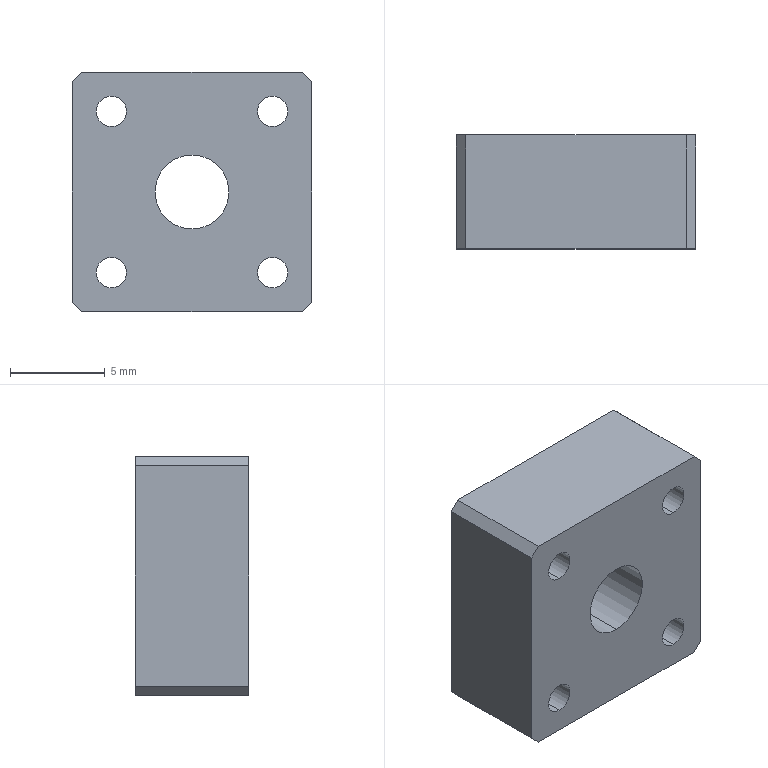Part | SolidWorks | features Extrusion 1, HoleWzd 1 | 1 solid | 20 faces | box 12.63 x 6 x 12.63 mm | volume 834.171 mm3 | cylinder 10 | plane 10 | commonest cylinder face diameters 1.6 x8 3.9 x2
STEP:
#1=CARTESIAN_POINT('',(-4.25,0.,-5.05));
#2=VERTEX_POINT('',#1);
#3=CARTESIAN_POINT('',(-4.25,0.,-3.45));
#4=VERTEX_POINT('',#3);
#5=CARTESIAN_POINT('',(-4.25,0.,-4.25));
#6=DIRECTION('',(0.,1.,0.));
#7=DIRECTION('',(0.,0.,1.));
#8=AXIS2_PLACEMENT_3D('',#5,#6,#7);
#9=CIRCLE('',#8,0.8);
#10=EDGE_CURVE('',#2,#4,#9,.T.);
#11=ORIENTED_EDGE('',*,*,#10,.F.);
#12=CARTESIAN_POINT('',(-4.25,6.,-5.05));
#13=VERTEX_POINT('',#12);
#14=CARTESIAN_POINT('',(-4.25,6.,-5.05));
#15=DIRECTION('',(0.,1.,0.));
#16=VECTOR('',#15,1000.);
#17=LINE('',#14,#16);
#18=EDGE_CURVE('',#2,#13,#17,.T.);
#19=ORIENTED_EDGE('',*,*,#18,.T.);
#20=CARTESIAN_POINT('',(-4.25,6.,-3.45));
#21=VERTEX_POINT('',#20);
#22=CARTESIAN_POINT('',(-4.25,6.,-4.25));
#23=DIRECTION('',(0.,1.,0.));
#24=DIRECTION('',(0.,0.,1.));
#25=AXIS2_PLACEMENT_3D('',#22,#23,#24);
#26=CIRCLE('',#25,0.8);
#27=EDGE_CURVE('',#13,#21,#26,.T.);
#28=ORIENTED_EDGE('',*,*,#27,.T.);
#29=CARTESIAN_POINT('',(-4.25,6.,-3.45));
#30=DIRECTION('',(0.,1.,0.));
#31=VECTOR('',#30,1000.);
#32=LINE('',#29,#31);
#33=EDGE_CURVE('',#4,#21,#32,.T.);
#34=ORIENTED_EDGE('',*,*,#33,.F.);
#35=EDGE_LOOP('',(#11,#19,#28,#34));
#36=FACE_OUTER_BOUND('',#35,.T.);
#37=CARTESIAN_POINT('',(-4.25,6.,-4.25));
#38=DIRECTION('',(0.,1.,0.));
#39=DIRECTION('',(0.,0.,1.));
#40=AXIS2_PLACEMENT_3D('',#37,#38,#39);
#41=CYLINDRICAL_SURFACE('',#40,0.8);
#42=ADVANCED_FACE('',(#36),#41,.F.);
#43=CARTESIAN_POINT('',(4.25,0.,-5.05));
#44=VERTEX_POINT('',#43);
#45=CARTESIAN_POINT('',(4.25,0.,-3.45));
#46=VERTEX_POINT('',#45);
#47=CARTESIAN_POINT('',(4.25,0.,-4.25));
#48=DIRECTION('',(0.,1.,0.));
#49=DIRECTION('',(0.,0.,1.));
#50=AXIS2_PLACEMENT_3D('',#47,#48,#49);
#51=CIRCLE('',#50,0.8);
#52=EDGE_CURVE('',#44,#46,#51,.T.);
#53=ORIENTED_EDGE('',*,*,#52,.F.);
#54=CARTESIAN_POINT('',(4.25,6.,-5.05));
#55=VERTEX_POINT('',#54);
#56=CARTESIAN_POINT('',(4.25,6.,-5.05));
#57=DIRECTION('',(0.,1.,0.));
#58=VECTOR('',#57,1000.);
#59=LINE('',#56,#58);
#60=EDGE_CURVE('',#44,#55,#59,.T.);
#61=ORIENTED_EDGE('',*,*,#60,.T.);
#62=CARTESIAN_POINT('',(4.25,6.,-3.45));
#63=VERTEX_POINT('',#62);
#64=CARTESIAN_POINT('',(4.25,6.,-4.25));
#65=DIRECTION('',(0.,1.,0.));
#66=DIRECTION('',(0.,0.,1.));
#67=AXIS2_PLACEMENT_3D('',#64,#65,#66);
#68=CIRCLE('',#67,0.8);
#69=EDGE_CURVE('',#55,#63,#68,.T.);
#70=ORIENTED_EDGE('',*,*,#69,.T.);
#71=CARTESIAN_POINT('',(4.25,6.,-3.45));
#72=DIRECTION('',(0.,1.,0.));
#73=VECTOR('',#72,1000.);
#74=LINE('',#71,#73);
#75=EDGE_CURVE('',#46,#63,#74,.T.);
#76=ORIENTED_EDGE('',*,*,#75,.F.);
#77=EDGE_LOOP('',(#53,#61,#70,#76));
#78=FACE_OUTER_BOUND('',#77,.T.);
#79=CARTESIAN_POINT('',(4.25,6.,-4.25));
#80=DIRECTION('',(0.,1.,0.));
#81=DIRECTION('',(0.,0.,1.));
#82=AXIS2_PLACEMENT_3D('',#79,#80,#81);
#83=CYLINDRICAL_SURFACE('',#82,0.8);
#84=ADVANCED_FACE('',(#78),#83,.F.);
#85=CARTESIAN_POINT('',(4.25,0.,3.45));
#86=VERTEX_POINT('',#85);
#87=CARTESIAN_POINT('',(4.25,0.,5.05));
#88=VERTEX_POINT('',#87);
#89=CARTESIAN_POINT('',(4.25,0.,4.25));
#90=DIRECTION('',(0.,1.,0.));
#91=DIRECTION('',(0.,0.,1.));
#92=AXIS2_PLACEMENT_3D('',#89,#90,#91);
#93=CIRCLE('',#92,0.8);
#94=EDGE_CURVE('',#86,#88,#93,.T.);
#95=ORIENTED_EDGE('',*,*,#94,.F.);
#96=CARTESIAN_POINT('',(4.25,6.,3.45));
#97=VERTEX_POINT('',#96);
#98=CARTESIAN_POINT('',(4.25,6.,3.45));
#99=DIRECTION('',(0.,1.,0.));
#100=VECTOR('',#99,1000.);
#101=LINE('',#98,#100);
#102=EDGE_CURVE('',#86,#97,#101,.T.);
#103=ORIENTED_EDGE('',*,*,#102,.T.);
#104=CARTESIAN_POINT('',(4.25,6.,5.05));
#105=VERTEX_POINT('',#104);
#106=CARTESIAN_POINT('',(4.25,6.,4.25));
#107=DIRECTION('',(0.,1.,0.));
#108=DIRECTION('',(0.,0.,1.));
#109=AXIS2_PLACEMENT_3D('',#106,#107,#108);
#110=CIRCLE('',#109,0.8);
#111=EDGE_CURVE('',#97,#105,#110,.T.);
#112=ORIENTED_EDGE('',*,*,#111,.T.);
#113=CARTESIAN_POINT('',(4.25,6.,5.05));
#114=DIRECTION('',(0.,1.,0.));
#115=VECTOR('',#114,1000.);
#116=LINE('',#113,#115);
#117=EDGE_CURVE('',#88,#105,#116,.T.);
#118=ORIENTED_EDGE('',*,*,#117,.F.);
#119=EDGE_LOOP('',(#95,#103,#112,#118));
#120=FACE_OUTER_BOUND('',#119,.T.);
#121=CARTESIAN_POINT('',(4.25,6.,4.25));
#122=DIRECTION('',(0.,1.,0.));
#123=DIRECTION('',(0.,0.,1.));
#124=AXIS2_PLACEMENT_3D('',#121,#122,#123);
#125=CYLINDRICAL_SURFACE('',#124,0.8);
#126=ADVANCED_FACE('',(#120),#125,.F.);
#127=CARTESIAN_POINT('',(-4.25,0.,3.45));
#128=VERTEX_POINT('',#127);
#129=CARTESIAN_POINT('',(-4.25,0.,5.05));
#130=VERTEX_POINT('',#129);
#131=CARTESIAN_POINT('',(-4.25,0.,4.25));
#132=DIRECTION('',(0.,1.,0.));
#133=DIRECTION('',(0.,0.,1.));
#134=AXIS2_PLACEMENT_3D('',#131,#132,#133);
#135=CIRCLE('',#134,0.8);
#136=EDGE_CURVE('',#128,#130,#135,.T.);
#137=ORIENTED_EDGE('',*,*,#136,.F.);
#138=CARTESIAN_POINT('',(-4.25,6.,3.45));
#139=VERTEX_POINT('',#138);
#140=CARTESIAN_POINT('',(-4.25,6.,3.45));
#141=DIRECTION('',(0.,1.,0.));
#142=VECTOR('',#141,1000.);
#143=LINE('',#140,#142);
#144=EDGE_CURVE('',#128,#139,#143,.T.);
#145=ORIENTED_EDGE('',*,*,#144,.T.);
#146=CARTESIAN_POINT('',(-4.25,6.,5.05));
#147=VERTEX_POINT('',#146);
#148=CARTESIAN_POINT('',(-4.25,6.,4.25));
#149=DIRECTION('',(0.,1.,0.));
#150=DIRECTION('',(0.,0.,1.));
#151=AXIS2_PLACEMENT_3D('',#148,#149,#150);
#152=CIRCLE('',#151,0.8);
#153=EDGE_CURVE('',#139,#147,#152,.T.);
#154=ORIENTED_EDGE('',*,*,#153,.T.);
#155=CARTESIAN_POINT('',(-4.25,6.,5.05));
#156=DIRECTION('',(0.,1.,0.));
#157=VECTOR('',#156,1000.);
#158=LINE('',#155,#157);
#159=EDGE_CURVE('',#130,#147,#158,.T.);
#160=ORIENTED_EDGE('',*,*,#159,.F.);
#161=EDGE_LOOP('',(#137,#145,#154,#160));
#162=FACE_OUTER_BOUND('',#161,.T.);
#163=CARTESIAN_POINT('',(-4.25,6.,4.25));
#164=DIRECTION('',(0.,1.,0.));
#165=DIRECTION('',(0.,0.,1.));
#166=AXIS2_PLACEMENT_3D('',#163,#164,#165);
#167=CYLINDRICAL_SURFACE('',#166,0.8);
#168=ADVANCED_FACE('',(#162),#167,.F.);
#169=CARTESIAN_POINT('',(0.,6.,-1.95));
#170=VERTEX_POINT('',#169);
#171=CARTESIAN_POINT('',(0.,6.,1.95));
#172=VERTEX_POINT('',#171);
#173=CARTESIAN_POINT('',(0.,6.,0.));
#174=DIRECTION('',(0.,1.,0.));
#175=DIRECTION('',(0.,0.,1.));
#176=AXIS2_PLACEMENT_3D('',#173,#174,#175);
#177=CIRCLE('',#176,1.95);
#178=EDGE_CURVE('',#170,#172,#177,.T.);
#179=ORIENTED_EDGE('',*,*,#178,.T.);
#180=CARTESIAN_POINT('',(0.,0.,1.95));
#181=VERTEX_POINT('',#180);
#182=CARTESIAN_POINT('',(0.,6.,1.95));
#183=DIRECTION('',(0.,-1.,0.));
#184=VECTOR('',#183,1000.);
#185=LINE('',#182,#184);
#186=EDGE_CURVE('',#172,#181,#185,.T.);
#187=ORIENTED_EDGE('',*,*,#186,.T.);
#188=CARTESIAN_POINT('',(0.,0.,-1.95));
#189=VERTEX_POINT('',#188);
#190=CARTESIAN_POINT('',(0.,0.,0.));
#191=DIRECTION('',(0.,1.,0.));
#192=DIRECTION('',(0.,0.,1.));
#193=AXIS2_PLACEMENT_3D('',#190,#191,#192);
#194=CIRCLE('',#193,1.95);
#195=EDGE_CURVE('',#189,#181,#194,.T.);
#196=ORIENTED_EDGE('',*,*,#195,.F.);
#197=CARTESIAN_POINT('',(0.,6.,-1.95));
#198=DIRECTION('',(0.,-1.,0.));
#199=VECTOR('',#198,1000.);
#200=LINE('',#197,#199);
#201=EDGE_CURVE('',#170,#189,#200,.T.);
#202=ORIENTED_EDGE('',*,*,#201,.F.);
#203=EDGE_LOOP('',(#179,#187,#196,#202));
#204=FACE_OUTER_BOUND('',#203,.T.);
#205=CARTESIAN_POINT('',(0.,6.,0.));
#206=DIRECTION('',(0.,-1.,0.));
#207=DIRECTION('',(0.,0.,-1.));
#208=AXIS2_PLACEMENT_3D('',#205,#206,#207);
#209=CYLINDRICAL_SURFACE('',#208,1.95);
#210=ADVANCED_FACE('',(#204),#209,.F.);
#211=CARTESIAN_POINT('',(-4.25,6.,-4.25));
#212=DIRECTION('',(0.,1.,0.));
#213=DIRECTION('',(0.,0.,1.));
#214=AXIS2_PLACEMENT_3D('',#211,#212,#213);
#215=CIRCLE('',#214,0.8);
#216=EDGE_CURVE('',#21,#13,#215,.T.);
#217=ORIENTED_EDGE('',*,*,#216,.F.);
#218=ORIENTED_EDGE('',*,*,#27,.F.);
#219=EDGE_LOOP('',(#217,#218));
#220=FACE_BOUND('',#219,.T.);
#221=CARTESIAN_POINT('',(4.25,6.,-4.25));
#222=DIRECTION('',(0.,1.,0.));
#223=DIRECTION('',(0.,0.,1.));
#224=AXIS2_PLACEMENT_3D('',#221,#222,#223);
#225=CIRCLE('',#224,0.8);
#226=EDGE_CURVE('',#63,#55,#225,.T.);
#227=ORIENTED_EDGE('',*,*,#226,.F.);
#228=ORIENTED_EDGE('',*,*,#69,.F.);
#229=EDGE_LOOP('',(#227,#228));
#230=FACE_BOUND('',#229,.T.);
#231=CARTESIAN_POINT('',(4.25,6.,4.25));
#232=DIRECTION('',(0.,1.,0.));
#233=DIRECTION('',(0.,0.,1.));
#234=AXIS2_PLACEMENT_3D('',#231,#232,#233);
#235=CIRCLE('',#234,0.8);
#236=EDGE_CURVE('',#105,#97,#235,.T.);
#237=ORIENTED_EDGE('',*,*,#236,.F.);
#238=ORIENTED_EDGE('',*,*,#111,.F.);
#239=EDGE_LOOP('',(#237,#238));
#240=FACE_BOUND('',#239,.T.);
#241=CARTESIAN_POINT('',(-4.25,6.,4.25));
#242=DIRECTION('',(0.,1.,0.));
#243=DIRECTION('',(0.,0.,1.));
#244=AXIS2_PLACEMENT_3D('',#241,#242,#243);
#245=CIRCLE('',#244,0.8);
#246=EDGE_CURVE('',#147,#139,#245,.T.);
#247=ORIENTED_EDGE('',*,*,#246,.F.);
#248=ORIENTED_EDGE('',*,*,#153,.F.);
#249=EDGE_LOOP('',(#247,#248));
#250=FACE_BOUND('',#249,.T.);
#251=CARTESIAN_POINT('',(-6.315,6.,-5.815));
#252=VERTEX_POINT('',#251);
#253=CARTESIAN_POINT('',(-6.315,6.,5.815));
#254=VERTEX_POINT('',#253);
#255=CARTESIAN_POINT('',(-6.315,6.,5.815));
#256=DIRECTION('',(0.,0.,1.));
#257=VECTOR('',#256,1000.);
#258=LINE('',#255,#257);
#259=EDGE_CURVE('',#252,#254,#258,.T.);
#260=ORIENTED_EDGE('',*,*,#259,.T.);
#261=CARTESIAN_POINT('',(-5.815,6.,6.315));
#262=VERTEX_POINT('',#261);
#263=CARTESIAN_POINT('',(-6.315,6.,5.815));
#264=DIRECTION('',(0.7071,0.,0.7071));
#265=VECTOR('',#264,1000.);
#266=LINE('',#263,#265);
#267=EDGE_CURVE('',#254,#262,#266,.T.);
#268=ORIENTED_EDGE('',*,*,#267,.T.);
#269=CARTESIAN_POINT('',(5.815,6.,6.315));
#270=VERTEX_POINT('',#269);
#271=CARTESIAN_POINT('',(-5.815,6.,6.315));
#272=DIRECTION('',(1.,0.,0.));
#273=VECTOR('',#272,1000.);
#274=LINE('',#271,#273);
#275=EDGE_CURVE('',#262,#270,#274,.T.);
#276=ORIENTED_EDGE('',*,*,#275,.T.);
#277=CARTESIAN_POINT('',(6.315,6.,5.815));
#278=VERTEX_POINT('',#277);
#279=CARTESIAN_POINT('',(5.815,6.,6.315));
#280=DIRECTION('',(0.7071,0.,-0.7071));
#281=VECTOR('',#280,1000.);
#282=LINE('',#279,#281);
#283=EDGE_CURVE('',#270,#278,#282,.T.);
#284=ORIENTED_EDGE('',*,*,#283,.T.);
#285=CARTESIAN_POINT('',(6.315,6.,-5.815));
#286=VERTEX_POINT('',#285);
#287=CARTESIAN_POINT('',(6.315,6.,5.815));
#288=DIRECTION('',(0.,0.,-1.));
#289=VECTOR('',#288,1000.);
#290=LINE('',#287,#289);
#291=EDGE_CURVE('',#278,#286,#290,.T.);
#292=ORIENTED_EDGE('',*,*,#291,.T.);
#293=CARTESIAN_POINT('',(5.815,6.,-6.315));
#294=VERTEX_POINT('',#293);
#295=CARTESIAN_POINT('',(5.815,6.,-6.315));
#296=DIRECTION('',(-0.7071,0.,-0.7071));
#297=VECTOR('',#296,1000.);
#298=LINE('',#295,#297);
#299=EDGE_CURVE('',#286,#294,#298,.T.);
#300=ORIENTED_EDGE('',*,*,#299,.T.);
#301=CARTESIAN_POINT('',(-5.815,6.,-6.315));
#302=VERTEX_POINT('',#301);
#303=CARTESIAN_POINT('',(-5.815,6.,-6.315));
#304=DIRECTION('',(-1.,0.,0.));
#305=VECTOR('',#304,1000.);
#306=LINE('',#303,#305);
#307=EDGE_CURVE('',#294,#302,#306,.T.);
#308=ORIENTED_EDGE('',*,*,#307,.T.);
#309=CARTESIAN_POINT('',(-6.315,6.,-5.815));
#310=DIRECTION('',(-0.7071,0.,0.7071));
#311=VECTOR('',#310,1000.);
#312=LINE('',#309,#311);
#313=EDGE_CURVE('',#302,#252,#312,.T.);
#314=ORIENTED_EDGE('',*,*,#313,.T.);
#315=EDGE_LOOP('',(#260,#268,#276,#284,#292,#300,#308,#314));
#316=FACE_OUTER_BOUND('',#315,.T.);
#317=ORIENTED_EDGE('',*,*,#178,.F.);
#318=CARTESIAN_POINT('',(0.,6.,0.));
#319=DIRECTION('',(0.,1.,0.));
#320=DIRECTION('',(0.,0.,1.));
#321=AXIS2_PLACEMENT_3D('',#318,#319,#320);
#322=CIRCLE('',#321,1.95);
#323=EDGE_CURVE('',#172,#170,#322,.T.);
#324=ORIENTED_EDGE('',*,*,#323,.F.);
#325=EDGE_LOOP('',(#317,#324));
#326=FACE_BOUND('',#325,.T.);
#327=CARTESIAN_POINT('',(-6.315,6.,-6.315));
#328=DIRECTION('',(0.,-1.,0.));
#329=DIRECTION('',(0.,0.,-1.));
#330=AXIS2_PLACEMENT_3D('',#327,#328,#329);
#331=PLANE('',#330);
#332=ADVANCED_FACE('',(#220,#230,#240,#250,#316,#326),#331,.F.);
#333=CARTESIAN_POINT('',(-4.25,0.,-4.25));
#334=DIRECTION('',(0.,1.,0.));
#335=DIRECTION('',(0.,0.,1.));
#336=AXIS2_PLACEMENT_3D('',#333,#334,#335);
#337=CIRCLE('',#336,0.8);
#338=EDGE_CURVE('',#4,#2,#337,.T.);
#339=ORIENTED_EDGE('',*,*,#338,.T.);
#340=ORIENTED_EDGE('',*,*,#10,.T.);
#341=EDGE_LOOP('',(#339,#340));
#342=FACE_BOUND('',#341,.T.);
#343=CARTESIAN_POINT('',(4.25,0.,-4.25));
#344=DIRECTION('',(0.,1.,0.));
#345=DIRECTION('',(0.,0.,1.));
#346=AXIS2_PLACEMENT_3D('',#343,#344,#345);
#347=CIRCLE('',#346,0.8);
#348=EDGE_CURVE('',#46,#44,#347,.T.);
#349=ORIENTED_EDGE('',*,*,#348,.T.);
#350=ORIENTED_EDGE('',*,*,#52,.T.);
#351=EDGE_LOOP('',(#349,#350));
#352=FACE_BOUND('',#351,.T.);
#353=CARTESIAN_POINT('',(4.25,0.,4.25));
#354=DIRECTION('',(0.,1.,0.));
#355=DIRECTION('',(0.,0.,1.));
#356=AXIS2_PLACEMENT_3D('',#353,#354,#355);
#357=CIRCLE('',#356,0.8);
#358=EDGE_CURVE('',#88,#86,#357,.T.);
#359=ORIENTED_EDGE('',*,*,#358,.T.);
#360=ORIENTED_EDGE('',*,*,#94,.T.);
#361=EDGE_LOOP('',(#359,#360));
#362=FACE_BOUND('',#361,.T.);
#363=CARTESIAN_POINT('',(-4.25,0.,4.25));
#364=DIRECTION('',(0.,1.,0.));
#365=DIRECTION('',(0.,0.,1.));
#366=AXIS2_PLACEMENT_3D('',#363,#364,#365);
#367=CIRCLE('',#366,0.8);
#368=EDGE_CURVE('',#130,#128,#367,.T.);
#369=ORIENTED_EDGE('',*,*,#368,.T.);
#370=ORIENTED_EDGE('',*,*,#136,.T.);
#371=EDGE_LOOP('',(#369,#370));
#372=FACE_BOUND('',#371,.T.);
#373=CARTESIAN_POINT('',(-6.315,0.,-5.815));
#374=VERTEX_POINT('',#373);
#375=CARTESIAN_POINT('',(-6.315,0.,5.815));
#376=VERTEX_POINT('',#375);
#377=CARTESIAN_POINT('',(-6.315,0.,5.815));
#378=DIRECTION('',(0.,0.,1.));
#379=VECTOR('',#378,1000.);
#380=LINE('',#377,#379);
#381=EDGE_CURVE('',#374,#376,#380,.T.);
#382=ORIENTED_EDGE('',*,*,#381,.F.);
#383=CARTESIAN_POINT('',(-5.815,0.,-6.315));
#384=VERTEX_POINT('',#383);
#385=CARTESIAN_POINT('',(-6.315,0.,-5.815));
#386=DIRECTION('',(-0.7071,0.,0.7071));
#387=VECTOR('',#386,1000.);
#388=LINE('',#385,#387);
#389=EDGE_CURVE('',#384,#374,#388,.T.);
#390=ORIENTED_EDGE('',*,*,#389,.F.);
#391=CARTESIAN_POINT('',(5.815,0.,-6.315));
#392=VERTEX_POINT('',#391);
#393=CARTESIAN_POINT('',(-5.815,0.,-6.315));
#394=DIRECTION('',(-1.,0.,0.));
#395=VECTOR('',#394,1000.);
#396=LINE('',#393,#395);
#397=EDGE_CURVE('',#392,#384,#396,.T.);
#398=ORIENTED_EDGE('',*,*,#397,.F.);
#399=CARTESIAN_POINT('',(6.315,0.,-5.815));
#400=VERTEX_POINT('',#399);
#401=CARTESIAN_POINT('',(5.815,0.,-6.315));
#402=DIRECTION('',(-0.7071,0.,-0.7071));
#403=VECTOR('',#402,1000.);
#404=LINE('',#401,#403);
#405=EDGE_CURVE('',#400,#392,#404,.T.);
#406=ORIENTED_EDGE('',*,*,#405,.F.);
#407=CARTESIAN_POINT('',(6.315,0.,5.815));
#408=VERTEX_POINT('',#407);
#409=CARTESIAN_POINT('',(6.315,0.,5.815));
#410=DIRECTION('',(0.,0.,-1.));
#411=VECTOR('',#410,1000.);
#412=LINE('',#409,#411);
#413=EDGE_CURVE('',#408,#400,#412,.T.);
#414=ORIENTED_EDGE('',*,*,#413,.F.);
#415=CARTESIAN_POINT('',(5.815,0.,6.315));
#416=VERTEX_POINT('',#415);
#417=CARTESIAN_POINT('',(5.815,0.,6.315));
#418=DIRECTION('',(0.7071,0.,-0.7071));
#419=VECTOR('',#418,1000.);
#420=LINE('',#417,#419);
#421=EDGE_CURVE('',#416,#408,#420,.T.);
#422=ORIENTED_EDGE('',*,*,#421,.F.);
#423=CARTESIAN_POINT('',(-5.815,0.,6.315));
#424=VERTEX_POINT('',#423);
#425=CARTESIAN_POINT('',(-5.815,0.,6.315));
#426=DIRECTION('',(1.,0.,0.));
#427=VECTOR('',#426,1000.);
#428=LINE('',#425,#427);
#429=EDGE_CURVE('',#424,#416,#428,.T.);
#430=ORIENTED_EDGE('',*,*,#429,.F.);
#431=CARTESIAN_POINT('',(-6.315,0.,5.815));
#432=DIRECTION('',(0.7071,0.,0.7071));
#433=VECTOR('',#432,1000.);
#434=LINE('',#431,#433);
#435=EDGE_CURVE('',#376,#424,#434,.T.);
#436=ORIENTED_EDGE('',*,*,#435,.F.);
#437=EDGE_LOOP('',(#382,#390,#398,#406,#414,#422,#430,#436));
#438=FACE_OUTER_BOUND('',#437,.T.);
#439=ORIENTED_EDGE('',*,*,#195,.T.);
#440=CARTESIAN_POINT('',(0.,0.,0.));
#441=DIRECTION('',(0.,1.,0.));
#442=DIRECTION('',(0.,0.,1.));
#443=AXIS2_PLACEMENT_3D('',#440,#441,#442);
#444=CIRCLE('',#443,1.95);
#445=EDGE_CURVE('',#181,#189,#444,.T.);
#446=ORIENTED_EDGE('',*,*,#445,.T.);
#447=EDGE_LOOP('',(#439,#446));
#448=FACE_BOUND('',#447,.T.);
#449=CARTESIAN_POINT('',(-6.315,0.,-6.315));
#450=DIRECTION('',(0.,-1.,0.));
#451=DIRECTION('',(0.,0.,-1.));
#452=AXIS2_PLACEMENT_3D('',#449,#450,#451);
#453=PLANE('',#452);
#454=ADVANCED_FACE('',(#342,#352,#362,#372,#438,#448),#453,.T.);
#455=ORIENTED_EDGE('',*,*,#381,.T.);
#456=CARTESIAN_POINT('',(-6.315,6.,5.815));
#457=DIRECTION('',(0.,-1.,0.));
#458=VECTOR('',#457,1000.);
#459=LINE('',#456,#458);
#460=EDGE_CURVE('',#254,#376,#459,.T.);
#461=ORIENTED_EDGE('',*,*,#460,.F.);
#462=ORIENTED_EDGE('',*,*,#259,.F.);
#463=CARTESIAN_POINT('',(-6.315,6.,-5.815));
#464=DIRECTION('',(0.,-1.,0.));
#465=VECTOR('',#464,1000.);
#466=LINE('',#463,#465);
#467=EDGE_CURVE('',#252,#374,#466,.T.);
#468=ORIENTED_EDGE('',*,*,#467,.T.);
#469=EDGE_LOOP('',(#455,#461,#462,#468));
#470=FACE_OUTER_BOUND('',#469,.T.);
#471=CARTESIAN_POINT('',(-6.315,6.,5.815));
#472=DIRECTION('',(1.,0.,0.));
#473=DIRECTION('',(0.,0.,-1.));
#474=AXIS2_PLACEMENT_3D('',#471,#472,#473);
#475=PLANE('',#474);
#476=ADVANCED_FACE('',(#470),#475,.F.);
#477=ORIENTED_EDGE('',*,*,#435,.T.);
#478=CARTESIAN_POINT('',(-5.815,6.,6.315));
#479=DIRECTION('',(0.,-1.,0.));
#480=VECTOR('',#479,1000.);
#481=LINE('',#478,#480);
#482=EDGE_CURVE('',#262,#424,#481,.T.);
#483=ORIENTED_EDGE('',*,*,#482,.F.);
#484=ORIENTED_EDGE('',*,*,#267,.F.);
#485=ORIENTED_EDGE('',*,*,#460,.T.);
#486=EDGE_LOOP('',(#477,#483,#484,#485));
#487=FACE_OUTER_BOUND('',#486,.T.);
#488=CARTESIAN_POINT('',(-6.315,6.,5.815));
#489=DIRECTION('',(0.7071,0.,-0.7071));
#490=DIRECTION('',(-0.7071,0.,-0.7071));
#491=AXIS2_PLACEMENT_3D('',#488,#489,#490);
#492=PLANE('',#491);
#493=ADVANCED_FACE('',(#487),#492,.F.);
#494=ORIENTED_EDGE('',*,*,#429,.T.);
#495=CARTESIAN_POINT('',(5.815,6.,6.315));
#496=DIRECTION('',(0.,-1.,0.));
#497=VECTOR('',#496,1000.);
#498=LINE('',#495,#497);
#499=EDGE_CURVE('',#270,#416,#498,.T.);
#500=ORIENTED_EDGE('',*,*,#499,.F.);
#501=ORIENTED_EDGE('',*,*,#275,.F.);
#502=ORIENTED_EDGE('',*,*,#482,.T.);
#503=EDGE_LOOP('',(#494,#500,#501,#502));
#504=FACE_OUTER_BOUND('',#503,.T.);
#505=CARTESIAN_POINT('',(-5.815,6.,6.315));
#506=DIRECTION('',(0.,0.,-1.));
#507=DIRECTION('',(-1.,0.,0.));
#508=AXIS2_PLACEMENT_3D('',#505,#506,#507);
#509=PLANE('',#508);
#510=ADVANCED_FACE('',(#504),#509,.F.);
#511=ORIENTED_EDGE('',*,*,#421,.T.);
#512=CARTESIAN_POINT('',(6.315,6.,5.815));
#513=DIRECTION('',(0.,-1.,0.));
#514=VECTOR('',#513,1000.);
#515=LINE('',#512,#514);
#516=EDGE_CURVE('',#278,#408,#515,.T.);
#517=ORIENTED_EDGE('',*,*,#516,.F.);
#518=ORIENTED_EDGE('',*,*,#283,.F.);
#519=ORIENTED_EDGE('',*,*,#499,.T.);
#520=EDGE_LOOP('',(#511,#517,#518,#519));
#521=FACE_OUTER_BOUND('',#520,.T.);
#522=CARTESIAN_POINT('',(5.815,6.,6.315));
#523=DIRECTION('',(-0.7071,0.,-0.7071));
#524=DIRECTION('',(-0.7071,0.,0.7071));
#525=AXIS2_PLACEMENT_3D('',#522,#523,#524);
#526=PLANE('',#525);
#527=ADVANCED_FACE('',(#521),#526,.F.);
#528=ORIENTED_EDGE('',*,*,#413,.T.);
#529=CARTESIAN_POINT('',(6.315,6.,-5.815));
#530=DIRECTION('',(0.,-1.,0.));
#531=VECTOR('',#530,1000.);
#532=LINE('',#529,#531);
#533=EDGE_CURVE('',#286,#400,#532,.T.);
#534=ORIENTED_EDGE('',*,*,#533,.F.);
#535=ORIENTED_EDGE('',*,*,#291,.F.);
#536=ORIENTED_EDGE('',*,*,#516,.T.);
#537=EDGE_LOOP('',(#528,#534,#535,#536));
#538=FACE_OUTER_BOUND('',#537,.T.);
#539=CARTESIAN_POINT('',(6.315,6.,5.815));
#540=DIRECTION('',(-1.,0.,0.));
#541=DIRECTION('',(0.,0.,1.));
#542=AXIS2_PLACEMENT_3D('',#539,#540,#541);
#543=PLANE('',#542);
#544=ADVANCED_FACE('',(#538),#543,.F.);
#545=ORIENTED_EDGE('',*,*,#405,.T.);
#546=CARTESIAN_POINT('',(5.815,6.,-6.315));
#547=DIRECTION('',(0.,-1.,0.));
#548=VECTOR('',#547,1000.);
#549=LINE('',#546,#548);
#550=EDGE_CURVE('',#294,#392,#549,.T.);
#551=ORIENTED_EDGE('',*,*,#550,.F.);
#552=ORIENTED_EDGE('',*,*,#299,.F.);
#553=ORIENTED_EDGE('',*,*,#533,.T.);
#554=EDGE_LOOP('',(#545,#551,#552,#553));
#555=FACE_OUTER_BOUND('',#554,.T.);
#556=CARTESIAN_POINT('',(5.815,6.,-6.315));
#557=DIRECTION('',(-0.7071,0.,0.7071));
#558=DIRECTION('',(0.7071,0.,0.7071));
#559=AXIS2_PLACEMENT_3D('',#556,#557,#558);
#560=PLANE('',#559);
#561=ADVANCED_FACE('',(#555),#560,.F.);
#562=ORIENTED_EDGE('',*,*,#397,.T.);
#563=CARTESIAN_POINT('',(-5.815,6.,-6.315));
#564=DIRECTION('',(0.,-1.,0.));
#565=VECTOR('',#564,1000.);
#566=LINE('',#563,#565);
#567=EDGE_CURVE('',#302,#384,#566,.T.);
#568=ORIENTED_EDGE('',*,*,#567,.F.);
#569=ORIENTED_EDGE('',*,*,#307,.F.);
#570=ORIENTED_EDGE('',*,*,#550,.T.);
#571=EDGE_LOOP('',(#562,#568,#569,#570));
#572=FACE_OUTER_BOUND('',#571,.T.);
#573=CARTESIAN_POINT('',(-5.815,6.,-6.315));
#574=DIRECTION('',(0.,0.,1.));
#575=DIRECTION('',(1.,0.,0.));
#576=AXIS2_PLACEMENT_3D('',#573,#574,#575);
#577=PLANE('',#576);
#578=ADVANCED_FACE('',(#572),#577,.F.);
#579=ORIENTED_EDGE('',*,*,#389,.T.);
#580=ORIENTED_EDGE('',*,*,#467,.F.);
#581=ORIENTED_EDGE('',*,*,#313,.F.);
#582=ORIENTED_EDGE('',*,*,#567,.T.);
#583=EDGE_LOOP('',(#579,#580,#581,#582));
#584=FACE_OUTER_BOUND('',#583,.T.);
#585=CARTESIAN_POINT('',(-6.315,6.,-5.815));
#586=DIRECTION('',(0.7071,0.,0.7071));
#587=DIRECTION('',(0.7071,0.,-0.7071));
#588=AXIS2_PLACEMENT_3D('',#585,#586,#587);
#589=PLANE('',#588);
#590=ADVANCED_FACE('',(#584),#589,.F.);
#591=ORIENTED_EDGE('',*,*,#186,.F.);
#592=ORIENTED_EDGE('',*,*,#323,.T.);
#593=ORIENTED_EDGE('',*,*,#201,.T.);
#594=ORIENTED_EDGE('',*,*,#445,.F.);
#595=EDGE_LOOP('',(#591,#592,#593,#594));
#596=FACE_OUTER_BOUND('',#595,.T.);
#597=CARTESIAN_POINT('',(0.,6.,0.));
#598=DIRECTION('',(0.,-1.,0.));
#599=DIRECTION('',(0.,0.,-1.));
#600=AXIS2_PLACEMENT_3D('',#597,#598,#599);
#601=CYLINDRICAL_SURFACE('',#600,1.95);
#602=ADVANCED_FACE('',(#596),#601,.F.);
#603=ORIENTED_EDGE('',*,*,#144,.F.);
#604=ORIENTED_EDGE('',*,*,#368,.F.);
#605=ORIENTED_EDGE('',*,*,#159,.T.);
#606=ORIENTED_EDGE('',*,*,#246,.T.);
#607=EDGE_LOOP('',(#603,#604,#605,#606));
#608=FACE_OUTER_BOUND('',#607,.T.);
#609=CARTESIAN_POINT('',(-4.25,6.,4.25));
#610=DIRECTION('',(0.,1.,0.));
#611=DIRECTION('',(0.,0.,1.));
#612=AXIS2_PLACEMENT_3D('',#609,#610,#611);
#613=CYLINDRICAL_SURFACE('',#612,0.8);
#614=ADVANCED_FACE('',(#608),#613,.F.);
#615=ORIENTED_EDGE('',*,*,#102,.F.);
#616=ORIENTED_EDGE('',*,*,#358,.F.);
#617=ORIENTED_EDGE('',*,*,#117,.T.);
#618=ORIENTED_EDGE('',*,*,#236,.T.);
#619=EDGE_LOOP('',(#615,#616,#617,#618));
#620=FACE_OUTER_BOUND('',#619,.T.);
#621=CARTESIAN_POINT('',(4.25,6.,4.25));
#622=DIRECTION('',(0.,1.,0.));
#623=DIRECTION('',(0.,0.,1.));
#624=AXIS2_PLACEMENT_3D('',#621,#622,#623);
#625=CYLINDRICAL_SURFACE('',#624,0.8);
#626=ADVANCED_FACE('',(#620),#625,.F.);
#627=ORIENTED_EDGE('',*,*,#60,.F.);
#628=ORIENTED_EDGE('',*,*,#348,.F.);
#629=ORIENTED_EDGE('',*,*,#75,.T.);
#630=ORIENTED_EDGE('',*,*,#226,.T.);
#631=EDGE_LOOP('',(#627,#628,#629,#630));
#632=FACE_OUTER_BOUND('',#631,.T.);
#633=CARTESIAN_POINT('',(4.25,6.,-4.25));
#634=DIRECTION('',(0.,1.,0.));
#635=DIRECTION('',(0.,0.,1.));
#636=AXIS2_PLACEMENT_3D('',#633,#634,#635);
#637=CYLINDRICAL_SURFACE('',#636,0.8);
#638=ADVANCED_FACE('',(#632),#637,.F.);
#639=ORIENTED_EDGE('',*,*,#18,.F.);
#640=ORIENTED_EDGE('',*,*,#338,.F.);
#641=ORIENTED_EDGE('',*,*,#33,.T.);
#642=ORIENTED_EDGE('',*,*,#216,.T.);
#643=EDGE_LOOP('',(#639,#640,#641,#642));
#644=FACE_OUTER_BOUND('',#643,.T.);
#645=CARTESIAN_POINT('',(-4.25,6.,-4.25));
#646=DIRECTION('',(0.,1.,0.));
#647=DIRECTION('',(0.,0.,1.));
#648=AXIS2_PLACEMENT_3D('',#645,#646,#647);
#649=CYLINDRICAL_SURFACE('',#648,0.8);
#650=ADVANCED_FACE('',(#644),#649,.F.);
#651=CLOSED_SHELL('',(#42,#84,#126,#168,#210,#332,#454,#476,#493,#510,#527,#544,#561,#578,#590,#602,#614,#626,#638,#650));
#652=MANIFOLD_SOLID_BREP('',#651);
#653=CARTESIAN_POINT('',(0.,0.,0.));
#654=DIRECTION('',(0.,0.,1.));
#655=DIRECTION('',(1.,0.,0.));
#656=AXIS2_PLACEMENT_3D('',#653,#654,#655);
#657=(LENGTH_UNIT()NAMED_UNIT(*)SI_UNIT(.MILLI.,.METRE.));
#658=UNCERTAINTY_MEASURE_WITH_UNIT(LENGTH_MEASURE(0.00001),#657,'','');
#659=(NAMED_UNIT(*)PLANE_ANGLE_UNIT()SI_UNIT($,.RADIAN.));
#660=(NAMED_UNIT(*)SI_UNIT($,.STERADIAN.)SOLID_ANGLE_UNIT());
#661=(GEOMETRIC_REPRESENTATION_CONTEXT(3)GLOBAL_UNCERTAINTY_ASSIGNED_CONTEXT((#658))GLOBAL_UNIT_ASSIGNED_CONTEXT((#657,#659,#660))REPRESENTATION_CONTEXT('',''));
#662=ADVANCED_BREP_SHAPE_REPRESENTATION('',(#652,#656),#661);